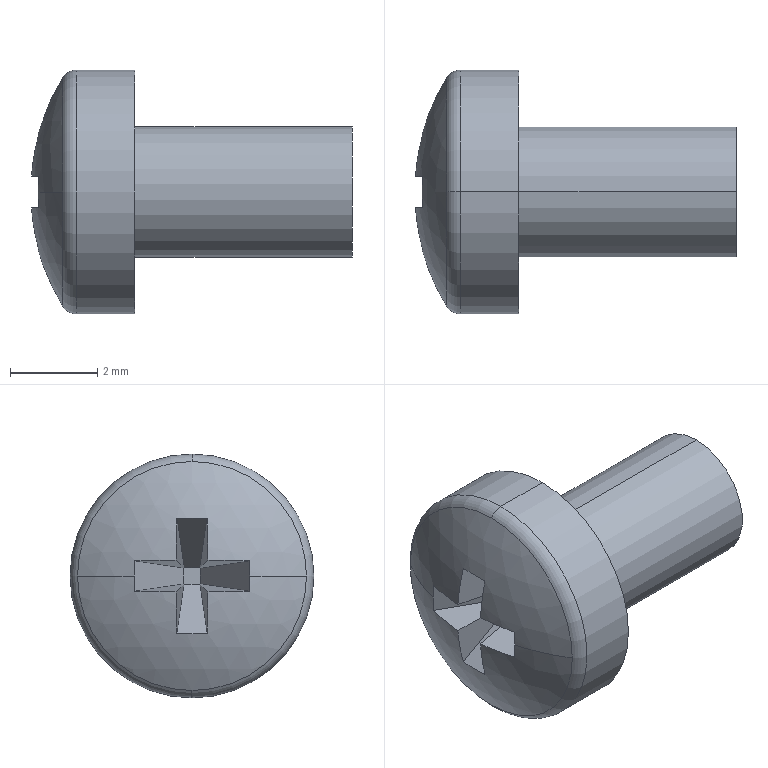Part | STEP file | B18.6.7M - M3 x 0.5 x 5 Type I Cross Recessed PHMS --5N | 1 solid | 23 faces | box 7.373 x 5.6 x 5.6 mm | volume 81.485 mm3 | plane 15 | cylinder 4 | torus 2 | sphere 2 | commonest cylinder face diameters 3 x2 5.6 x2